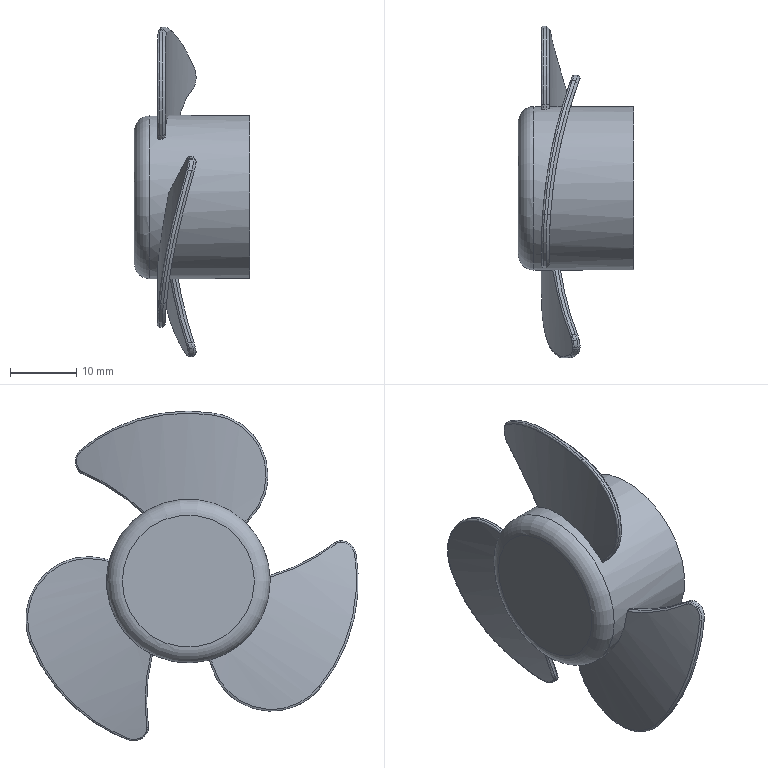Part | NX | features BREP 1 | 1 solid | 86 faces | box 17.486 x 50.35 x 49.901 mm | volume 9521 mm3 | spline 52 | cylinder 25 | plane 8 | torus 1 | commonest cylinder face diameters 4.762 x6 2.857 x3 19.048 x3 51.429 x3 58.887 x3 149.379 x3